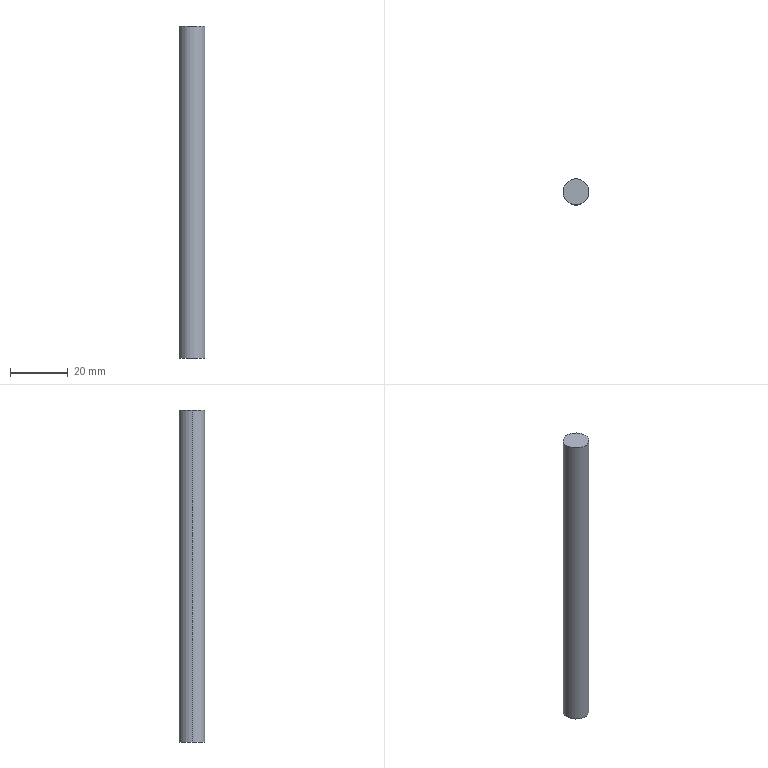Part | SolidWorks | features BaseBody 1 | 1 solid | 4 faces | box 9 x 9 x 115 mm | volume 7316 mm3 | cylinder 2 | plane 2 | commonest cylinder face diameters 9 x2
STEP:
#1=CARTESIAN_POINT('',(4.5,0.,-57.5));
#2=VERTEX_POINT('',#1);
#3=CARTESIAN_POINT('',(-4.5,0.,-57.5));
#4=VERTEX_POINT('',#3);
#5=CARTESIAN_POINT('',(0.,0.,-57.5));
#6=DIRECTION('',(0.,0.,1.));
#7=DIRECTION('',(1.,0.,0.));
#8=AXIS2_PLACEMENT_3D('',#5,#6,#7);
#9=CIRCLE('',#8,4.5);
#10=EDGE_CURVE('',#2,#4,#9,.T.);
#11=ORIENTED_EDGE('',*,*,#10,.T.);
#12=CARTESIAN_POINT('',(-4.5,0.,57.5));
#13=VERTEX_POINT('',#12);
#14=CARTESIAN_POINT('',(-4.5,0.,57.5));
#15=DIRECTION('',(0.,0.,1.));
#16=VECTOR('',#15,1000.);
#17=LINE('',#14,#16);
#18=EDGE_CURVE('',#4,#13,#17,.T.);
#19=ORIENTED_EDGE('',*,*,#18,.T.);
#20=CARTESIAN_POINT('',(4.5,0.,57.5));
#21=VERTEX_POINT('',#20);
#22=CARTESIAN_POINT('',(0.,0.,57.5));
#23=DIRECTION('',(0.,0.,-1.));
#24=DIRECTION('',(1.,0.,0.));
#25=AXIS2_PLACEMENT_3D('',#22,#23,#24);
#26=CIRCLE('',#25,4.5);
#27=EDGE_CURVE('',#13,#21,#26,.T.);
#28=ORIENTED_EDGE('',*,*,#27,.T.);
#29=CARTESIAN_POINT('',(4.5,0.,57.5));
#30=DIRECTION('',(0.,0.,1.));
#31=VECTOR('',#30,1000.);
#32=LINE('',#29,#31);
#33=EDGE_CURVE('',#2,#21,#32,.T.);
#34=ORIENTED_EDGE('',*,*,#33,.F.);
#35=EDGE_LOOP('',(#11,#19,#28,#34));
#36=FACE_OUTER_BOUND('',#35,.T.);
#37=CARTESIAN_POINT('',(0.,0.,57.5));
#38=DIRECTION('',(0.,0.,1.));
#39=DIRECTION('',(1.,0.,0.));
#40=AXIS2_PLACEMENT_3D('',#37,#38,#39);
#41=CYLINDRICAL_SURFACE('',#40,4.5);
#42=ADVANCED_FACE('',(#36),#41,.T.);
#43=ORIENTED_EDGE('',*,*,#18,.F.);
#44=CARTESIAN_POINT('',(0.,0.,-57.5));
#45=DIRECTION('',(0.,0.,1.));
#46=DIRECTION('',(1.,0.,0.));
#47=AXIS2_PLACEMENT_3D('',#44,#45,#46);
#48=CIRCLE('',#47,4.5);
#49=EDGE_CURVE('',#4,#2,#48,.T.);
#50=ORIENTED_EDGE('',*,*,#49,.T.);
#51=ORIENTED_EDGE('',*,*,#33,.T.);
#52=CARTESIAN_POINT('',(0.,0.,57.5));
#53=DIRECTION('',(0.,0.,-1.));
#54=DIRECTION('',(1.,0.,0.));
#55=AXIS2_PLACEMENT_3D('',#52,#53,#54);
#56=CIRCLE('',#55,4.5);
#57=EDGE_CURVE('',#21,#13,#56,.T.);
#58=ORIENTED_EDGE('',*,*,#57,.T.);
#59=EDGE_LOOP('',(#43,#50,#51,#58));
#60=FACE_OUTER_BOUND('',#59,.T.);
#61=CARTESIAN_POINT('',(0.,0.,57.5));
#62=DIRECTION('',(0.,0.,1.));
#63=DIRECTION('',(1.,0.,0.));
#64=AXIS2_PLACEMENT_3D('',#61,#62,#63);
#65=CYLINDRICAL_SURFACE('',#64,4.5);
#66=ADVANCED_FACE('',(#60),#65,.T.);
#67=ORIENTED_EDGE('',*,*,#57,.F.);
#68=ORIENTED_EDGE('',*,*,#27,.F.);
#69=EDGE_LOOP('',(#67,#68));
#70=FACE_OUTER_BOUND('',#69,.T.);
#71=CARTESIAN_POINT('',(0.,0.,57.5));
#72=DIRECTION('',(0.,0.,1.));
#73=DIRECTION('',(1.,0.,0.));
#74=AXIS2_PLACEMENT_3D('',#71,#72,#73);
#75=PLANE('',#74);
#76=ADVANCED_FACE('',(#70),#75,.T.);
#77=ORIENTED_EDGE('',*,*,#10,.F.);
#78=ORIENTED_EDGE('',*,*,#49,.F.);
#79=EDGE_LOOP('',(#77,#78));
#80=FACE_OUTER_BOUND('',#79,.T.);
#81=CARTESIAN_POINT('',(0.,0.,-57.5));
#82=DIRECTION('',(0.,0.,1.));
#83=DIRECTION('',(1.,0.,0.));
#84=AXIS2_PLACEMENT_3D('',#81,#82,#83);
#85=PLANE('',#84);
#86=ADVANCED_FACE('',(#80),#85,.F.);
#87=CLOSED_SHELL('',(#42,#66,#76,#86));
#88=MANIFOLD_SOLID_BREP('',#87);
#89=CARTESIAN_POINT('',(0.,0.,0.));
#90=DIRECTION('',(0.,0.,1.));
#91=DIRECTION('',(1.,0.,0.));
#92=AXIS2_PLACEMENT_3D('',#89,#90,#91);
#93=(LENGTH_UNIT()NAMED_UNIT(*)SI_UNIT(.MILLI.,.METRE.));
#94=UNCERTAINTY_MEASURE_WITH_UNIT(LENGTH_MEASURE(0.00001),#93,'','');
#95=(NAMED_UNIT(*)PLANE_ANGLE_UNIT()SI_UNIT($,.RADIAN.));
#96=(NAMED_UNIT(*)SI_UNIT($,.STERADIAN.)SOLID_ANGLE_UNIT());
#97=(GEOMETRIC_REPRESENTATION_CONTEXT(3)GLOBAL_UNCERTAINTY_ASSIGNED_CONTEXT((#94))GLOBAL_UNIT_ASSIGNED_CONTEXT((#93,#95,#96))REPRESENTATION_CONTEXT('',''));
#98=ADVANCED_BREP_SHAPE_REPRESENTATION('',(#88,#92),#97);